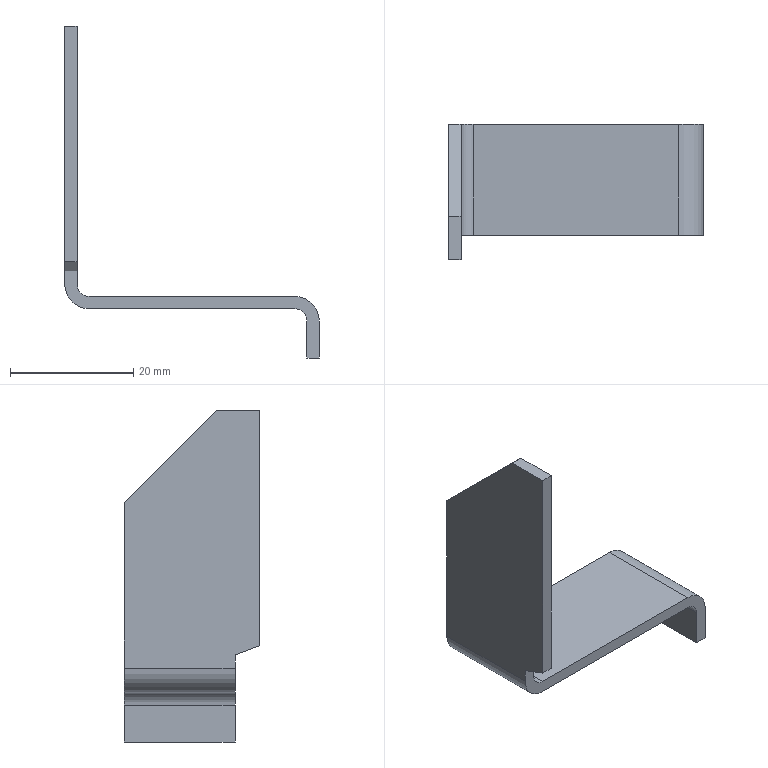Part | NX | features solid 2 | 1 solid | 17 faces | box 41.351 x 22 x 53.937 mm | volume 3353 mm3 | plane 13 | cylinder 4 | commonest cylinder face diameters 4 x2 8 x2
STEP:
#1=CARTESIAN_POINT('',(1112.,-1287.,212.));
#2=VERTEX_POINT('',#1);
#3=CARTESIAN_POINT('',(1112.,-1302.,227.));
#4=VERTEX_POINT('',#3);
#5=CARTESIAN_POINT('',(1112.,-1283.97,208.97));
#6=DIRECTION('',(0.,-0.7071,0.7071));
#7=VECTOR('',#6,1000.);
#8=LINE('',#5,#7);
#9=EDGE_CURVE('',#2,#4,#8,.T.);
#10=ORIENTED_EDGE('',*,*,#9,.F.);
#11=CARTESIAN_POINT('',(1110.,-1287.,212.));
#12=VERTEX_POINT('',#11);
#13=CARTESIAN_POINT('',(1112.,-1287.,212.));
#14=DIRECTION('',(1.,0.,0.));
#15=VECTOR('',#14,1000.);
#16=LINE('',#13,#15);
#17=EDGE_CURVE('',#12,#2,#16,.T.);
#18=ORIENTED_EDGE('',*,*,#17,.F.);
#19=CARTESIAN_POINT('',(1110.,-1302.,227.));
#20=VERTEX_POINT('',#19);
#21=CARTESIAN_POINT('',(1110.,-1302.,227.));
#22=DIRECTION('',(0.,0.7071,-0.7071));
#23=VECTOR('',#22,1000.);
#24=LINE('',#21,#23);
#25=EDGE_CURVE('',#20,#12,#24,.T.);
#26=ORIENTED_EDGE('',*,*,#25,.F.);
#27=CARTESIAN_POINT('',(1112.,-1302.,227.));
#28=DIRECTION('',(-1.,0.,0.));
#29=VECTOR('',#28,1000.);
#30=LINE('',#27,#29);
#31=EDGE_CURVE('',#4,#20,#30,.T.);
#32=ORIENTED_EDGE('',*,*,#31,.F.);
#33=EDGE_LOOP('',(#10,#18,#26,#32));
#34=FACE_BOUND('',#33,.T.);
#35=CARTESIAN_POINT('',(1112.,-1302.,227.));
#36=DIRECTION('',(0.,-0.7071,-0.7071));
#37=DIRECTION('',(0.,0.7071,-0.7071));
#38=AXIS2_PLACEMENT_3D('',#35,#36,#37);
#39=PLANE('',#38);
#40=ADVANCED_FACE('',(#34),#39,.F.);
#41=CARTESIAN_POINT('',(1147.351,-1287.,181.063));
#42=VERTEX_POINT('',#41);
#43=CARTESIAN_POINT('',(1149.351,-1287.,179.063));
#44=VERTEX_POINT('',#43);
#45=CARTESIAN_POINT('',(1147.351,-1287.,179.063));
#46=DIRECTION('',(0.,1.,0.));
#47=DIRECTION('',(0.,0.,1.));
#48=AXIS2_PLACEMENT_3D('',#45,#46,#47);
#49=CIRCLE('',#48,2.);
#50=EDGE_CURVE('',#42,#44,#49,.T.);
#51=ORIENTED_EDGE('',*,*,#50,.T.);
#52=CARTESIAN_POINT('',(1149.351,-1305.,179.063));
#53=VERTEX_POINT('',#52);
#54=CARTESIAN_POINT('',(1149.351,-1267.,179.063));
#55=DIRECTION('',(0.,-1.,0.));
#56=VECTOR('',#55,1000.);
#57=LINE('',#54,#56);
#58=EDGE_CURVE('',#44,#53,#57,.T.);
#59=ORIENTED_EDGE('',*,*,#58,.T.);
#60=CARTESIAN_POINT('',(1147.351,-1305.,181.063));
#61=VERTEX_POINT('',#60);
#62=CARTESIAN_POINT('',(1147.351,-1305.,179.063));
#63=DIRECTION('',(0.,-1.,0.));
#64=DIRECTION('',(0.,0.,1.));
#65=AXIS2_PLACEMENT_3D('',#62,#63,#64);
#66=CIRCLE('',#65,2.);
#67=EDGE_CURVE('',#53,#61,#66,.T.);
#68=ORIENTED_EDGE('',*,*,#67,.T.);
#69=CARTESIAN_POINT('',(1147.351,-1305.,181.063));
#70=DIRECTION('',(0.,1.,0.));
#71=VECTOR('',#70,1000.);
#72=LINE('',#69,#71);
#73=EDGE_CURVE('',#61,#42,#72,.T.);
#74=ORIENTED_EDGE('',*,*,#73,.T.);
#75=EDGE_LOOP('',(#51,#59,#68,#74));
#76=FACE_BOUND('',#75,.T.);
#77=CARTESIAN_POINT('',(1147.351,-1305.,179.063));
#78=DIRECTION('',(0.,1.,0.));
#79=DIRECTION('',(0.,0.,-1.));
#80=AXIS2_PLACEMENT_3D('',#77,#78,#79);
#81=CYLINDRICAL_SURFACE('',#80,2.);
#82=ADVANCED_FACE('',(#76),#81,.F.);
#83=CARTESIAN_POINT('',(1147.351,-1287.,183.063));
#84=VERTEX_POINT('',#83);
#85=CARTESIAN_POINT('',(1151.351,-1287.,179.063));
#86=VERTEX_POINT('',#85);
#87=CARTESIAN_POINT('',(1147.351,-1287.,179.063));
#88=DIRECTION('',(0.,1.,0.));
#89=DIRECTION('',(0.,0.,-1.));
#90=AXIS2_PLACEMENT_3D('',#87,#88,#89);
#91=CIRCLE('',#90,4.);
#92=EDGE_CURVE('',#84,#86,#91,.T.);
#93=ORIENTED_EDGE('',*,*,#92,.F.);
#94=CARTESIAN_POINT('',(1147.351,-1305.,183.063));
#95=VERTEX_POINT('',#94);
#96=CARTESIAN_POINT('',(1147.351,-1305.,183.063));
#97=DIRECTION('',(0.,1.,0.));
#98=VECTOR('',#97,1000.);
#99=LINE('',#96,#98);
#100=EDGE_CURVE('',#95,#84,#99,.T.);
#101=ORIENTED_EDGE('',*,*,#100,.F.);
#102=CARTESIAN_POINT('',(1151.351,-1305.,179.063));
#103=VERTEX_POINT('',#102);
#104=CARTESIAN_POINT('',(1147.351,-1305.,179.063));
#105=DIRECTION('',(0.,-1.,0.));
#106=DIRECTION('',(0.,0.,-1.));
#107=AXIS2_PLACEMENT_3D('',#104,#105,#106);
#108=CIRCLE('',#107,4.);
#109=EDGE_CURVE('',#103,#95,#108,.T.);
#110=ORIENTED_EDGE('',*,*,#109,.F.);
#111=CARTESIAN_POINT('',(1151.351,-1267.,179.063));
#112=DIRECTION('',(0.,-1.,0.));
#113=VECTOR('',#112,1000.);
#114=LINE('',#111,#113);
#115=EDGE_CURVE('',#86,#103,#114,.T.);
#116=ORIENTED_EDGE('',*,*,#115,.F.);
#117=EDGE_LOOP('',(#93,#101,#110,#116));
#118=FACE_BOUND('',#117,.T.);
#119=CARTESIAN_POINT('',(1147.351,-1305.,179.063));
#120=DIRECTION('',(0.,1.,0.));
#121=DIRECTION('',(0.,0.,-1.));
#122=AXIS2_PLACEMENT_3D('',#119,#120,#121);
#123=CYLINDRICAL_SURFACE('',#122,4.);
#124=ADVANCED_FACE('',(#118),#123,.T.);
#125=CARTESIAN_POINT('',(1149.351,-1305.,173.063));
#126=VERTEX_POINT('',#125);
#127=CARTESIAN_POINT('',(1149.351,-1287.,173.063));
#128=VERTEX_POINT('',#127);
#129=CARTESIAN_POINT('',(1149.351,-1305.,173.063));
#130=DIRECTION('',(0.,1.,0.));
#131=VECTOR('',#130,1000.);
#132=LINE('',#129,#131);
#133=EDGE_CURVE('',#126,#128,#132,.T.);
#134=ORIENTED_EDGE('',*,*,#133,.T.);
#135=CARTESIAN_POINT('',(1151.351,-1287.,173.063));
#136=VERTEX_POINT('',#135);
#137=CARTESIAN_POINT('',(1151.351,-1287.,173.063));
#138=DIRECTION('',(-1.,0.,0.));
#139=VECTOR('',#138,1000.);
#140=LINE('',#137,#139);
#141=EDGE_CURVE('',#136,#128,#140,.T.);
#142=ORIENTED_EDGE('',*,*,#141,.F.);
#143=CARTESIAN_POINT('',(1151.351,-1305.,173.063));
#144=VERTEX_POINT('',#143);
#145=CARTESIAN_POINT('',(1151.351,-1305.,173.063));
#146=DIRECTION('',(0.,1.,0.));
#147=VECTOR('',#146,1000.);
#148=LINE('',#145,#147);
#149=EDGE_CURVE('',#144,#136,#148,.T.);
#150=ORIENTED_EDGE('',*,*,#149,.F.);
#151=CARTESIAN_POINT('',(1151.351,-1305.,173.063));
#152=DIRECTION('',(-1.,0.,0.));
#153=VECTOR('',#152,1000.);
#154=LINE('',#151,#153);
#155=EDGE_CURVE('',#144,#126,#154,.T.);
#156=ORIENTED_EDGE('',*,*,#155,.T.);
#157=EDGE_LOOP('',(#134,#142,#150,#156));
#158=FACE_BOUND('',#157,.T.);
#159=CARTESIAN_POINT('',(1151.351,-1305.,173.063));
#160=DIRECTION('',(0.,0.,1.));
#161=DIRECTION('',(1.,0.,0.));
#162=AXIS2_PLACEMENT_3D('',#159,#160,#161);
#163=PLANE('',#162);
#164=ADVANCED_FACE('',(#158),#163,.F.);
#165=ORIENTED_EDGE('',*,*,#58,.F.);
#166=CARTESIAN_POINT('',(1149.351,-1287.,181.341));
#167=DIRECTION('',(0.,0.,1.));
#168=VECTOR('',#167,1000.);
#169=LINE('',#166,#168);
#170=EDGE_CURVE('',#128,#44,#169,.T.);
#171=ORIENTED_EDGE('',*,*,#170,.F.);
#172=ORIENTED_EDGE('',*,*,#133,.F.);
#173=CARTESIAN_POINT('',(1149.351,-1305.,181.341));
#174=DIRECTION('',(0.,0.,-1.));
#175=VECTOR('',#174,1000.);
#176=LINE('',#173,#175);
#177=EDGE_CURVE('',#53,#126,#176,.T.);
#178=ORIENTED_EDGE('',*,*,#177,.F.);
#179=EDGE_LOOP('',(#165,#171,#172,#178));
#180=FACE_BOUND('',#179,.T.);
#181=CARTESIAN_POINT('',(1149.351,-1555.,-62.061));
#182=DIRECTION('',(1.,0.,0.));
#183=DIRECTION('',(0.,0.,1.));
#184=AXIS2_PLACEMENT_3D('',#181,#182,#183);
#185=PLANE('',#184);
#186=ADVANCED_FACE('',(#180),#185,.F.);
#187=CARTESIAN_POINT('',(1151.351,-1287.,181.341));
#188=DIRECTION('',(0.,0.,1.));
#189=VECTOR('',#188,1000.);
#190=LINE('',#187,#189);
#191=EDGE_CURVE('',#136,#86,#190,.T.);
#192=ORIENTED_EDGE('',*,*,#191,.T.);
#193=ORIENTED_EDGE('',*,*,#115,.T.);
#194=CARTESIAN_POINT('',(1151.351,-1305.,181.341));
#195=DIRECTION('',(0.,0.,-1.));
#196=VECTOR('',#195,1000.);
#197=LINE('',#194,#196);
#198=EDGE_CURVE('',#103,#144,#197,.T.);
#199=ORIENTED_EDGE('',*,*,#198,.T.);
#200=ORIENTED_EDGE('',*,*,#149,.T.);
#201=EDGE_LOOP('',(#192,#193,#199,#200));
#202=FACE_BOUND('',#201,.T.);
#203=CARTESIAN_POINT('',(1151.351,-1555.,-62.061));
#204=DIRECTION('',(1.,0.,0.));
#205=DIRECTION('',(0.,0.,1.));
#206=AXIS2_PLACEMENT_3D('',#203,#204,#205);
#207=PLANE('',#206);
#208=ADVANCED_FACE('',(#202),#207,.T.);
#209=CARTESIAN_POINT('',(1112.,-1287.,185.063));
#210=VERTEX_POINT('',#209);
#211=CARTESIAN_POINT('',(1112.,-1305.,185.063));
#212=VERTEX_POINT('',#211);
#213=CARTESIAN_POINT('',(1112.,-1267.,185.063));
#214=DIRECTION('',(0.,-1.,0.));
#215=VECTOR('',#214,1000.);
#216=LINE('',#213,#215);
#217=EDGE_CURVE('',#210,#212,#216,.T.);
#218=ORIENTED_EDGE('',*,*,#217,.T.);
#219=CARTESIAN_POINT('',(1114.,-1305.,183.063));
#220=VERTEX_POINT('',#219);
#221=CARTESIAN_POINT('',(1114.,-1305.,185.063));
#222=DIRECTION('',(0.,-1.,0.));
#223=DIRECTION('',(0.,0.,-1.));
#224=AXIS2_PLACEMENT_3D('',#221,#222,#223);
#225=CIRCLE('',#224,2.);
#226=EDGE_CURVE('',#212,#220,#225,.T.);
#227=ORIENTED_EDGE('',*,*,#226,.T.);
#228=CARTESIAN_POINT('',(1114.,-1287.,183.063));
#229=VERTEX_POINT('',#228);
#230=CARTESIAN_POINT('',(1114.,-1305.,183.063));
#231=DIRECTION('',(0.,1.,0.));
#232=VECTOR('',#231,1000.);
#233=LINE('',#230,#232);
#234=EDGE_CURVE('',#220,#229,#233,.T.);
#235=ORIENTED_EDGE('',*,*,#234,.T.);
#236=CARTESIAN_POINT('',(1114.,-1287.,185.063));
#237=DIRECTION('',(0.,1.,0.));
#238=DIRECTION('',(0.,0.,-1.));
#239=AXIS2_PLACEMENT_3D('',#236,#237,#238);
#240=CIRCLE('',#239,2.);
#241=EDGE_CURVE('',#229,#210,#240,.T.);
#242=ORIENTED_EDGE('',*,*,#241,.T.);
#243=EDGE_LOOP('',(#218,#227,#235,#242));
#244=FACE_BOUND('',#243,.T.);
#245=CARTESIAN_POINT('',(1114.,-1267.,185.063));
#246=DIRECTION('',(0.,-1.,0.));
#247=DIRECTION('',(1.,0.,0.));
#248=AXIS2_PLACEMENT_3D('',#245,#246,#247);
#249=CYLINDRICAL_SURFACE('',#248,2.);
#250=ADVANCED_FACE('',(#244),#249,.F.);
#251=CARTESIAN_POINT('',(1110.,-1287.,185.063));
#252=VERTEX_POINT('',#251);
#253=CARTESIAN_POINT('',(1110.,-1305.,185.063));
#254=VERTEX_POINT('',#253);
#255=CARTESIAN_POINT('',(1110.,-1267.,185.063));
#256=DIRECTION('',(0.,-1.,0.));
#257=VECTOR('',#256,1000.);
#258=LINE('',#255,#257);
#259=EDGE_CURVE('',#252,#254,#258,.T.);
#260=ORIENTED_EDGE('',*,*,#259,.F.);
#261=CARTESIAN_POINT('',(1114.,-1287.,181.063));
#262=VERTEX_POINT('',#261);
#263=CARTESIAN_POINT('',(1114.,-1287.,185.063));
#264=DIRECTION('',(0.,1.,0.));
#265=DIRECTION('',(1.,0.,0.));
#266=AXIS2_PLACEMENT_3D('',#263,#264,#265);
#267=CIRCLE('',#266,4.);
#268=EDGE_CURVE('',#262,#252,#267,.T.);
#269=ORIENTED_EDGE('',*,*,#268,.F.);
#270=CARTESIAN_POINT('',(1114.,-1305.,181.063));
#271=VERTEX_POINT('',#270);
#272=CARTESIAN_POINT('',(1114.,-1305.,181.063));
#273=DIRECTION('',(0.,1.,0.));
#274=VECTOR('',#273,1000.);
#275=LINE('',#272,#274);
#276=EDGE_CURVE('',#271,#262,#275,.T.);
#277=ORIENTED_EDGE('',*,*,#276,.F.);
#278=CARTESIAN_POINT('',(1114.,-1305.,185.063));
#279=DIRECTION('',(0.,-1.,0.));
#280=DIRECTION('',(1.,0.,0.));
#281=AXIS2_PLACEMENT_3D('',#278,#279,#280);
#282=CIRCLE('',#281,4.);
#283=EDGE_CURVE('',#254,#271,#282,.T.);
#284=ORIENTED_EDGE('',*,*,#283,.F.);
#285=EDGE_LOOP('',(#260,#269,#277,#284));
#286=FACE_BOUND('',#285,.T.);
#287=CARTESIAN_POINT('',(1114.,-1267.,185.063));
#288=DIRECTION('',(0.,-1.,0.));
#289=DIRECTION('',(1.,0.,0.));
#290=AXIS2_PLACEMENT_3D('',#287,#288,#289);
#291=CYLINDRICAL_SURFACE('',#290,4.);
#292=ADVANCED_FACE('',(#286),#291,.T.);
#293=ORIENTED_EDGE('',*,*,#73,.F.);
#294=CARTESIAN_POINT('',(1111.722,-1305.,181.063));
#295=DIRECTION('',(-1.,0.,0.));
#296=VECTOR('',#295,1000.);
#297=LINE('',#294,#296);
#298=EDGE_CURVE('',#61,#271,#297,.T.);
#299=ORIENTED_EDGE('',*,*,#298,.T.);
#300=ORIENTED_EDGE('',*,*,#276,.T.);
#301=CARTESIAN_POINT('',(1111.722,-1287.,181.063));
#302=DIRECTION('',(1.,0.,0.));
#303=VECTOR('',#302,1000.);
#304=LINE('',#301,#303);
#305=EDGE_CURVE('',#262,#42,#304,.T.);
#306=ORIENTED_EDGE('',*,*,#305,.T.);
#307=EDGE_LOOP('',(#293,#299,#300,#306));
#308=FACE_BOUND('',#307,.T.);
#309=CARTESIAN_POINT('',(1110.,-1555.,181.063));
#310=DIRECTION('',(0.,0.,-1.));
#311=DIRECTION('',(0.,-1.,0.));
#312=AXIS2_PLACEMENT_3D('',#309,#310,#311);
#313=PLANE('',#312);
#314=ADVANCED_FACE('',(#308),#313,.T.);
#315=CARTESIAN_POINT('',(1112.,-1287.,227.));
#316=DIRECTION('',(0.,0.,1.));
#317=VECTOR('',#316,1000.);
#318=LINE('',#315,#317);
#319=EDGE_CURVE('',#210,#2,#318,.T.);
#320=ORIENTED_EDGE('',*,*,#319,.T.);
#321=ORIENTED_EDGE('',*,*,#9,.T.);
#322=CARTESIAN_POINT('',(1112.,-1309.,227.));
#323=VERTEX_POINT('',#322);
#324=CARTESIAN_POINT('',(1112.,-1309.,227.));
#325=DIRECTION('',(0.,-1.,0.));
#326=VECTOR('',#325,1000.);
#327=LINE('',#324,#326);
#328=EDGE_CURVE('',#4,#323,#327,.T.);
#329=ORIENTED_EDGE('',*,*,#328,.T.);
#330=CARTESIAN_POINT('',(1112.,-1309.,188.716));
#331=VERTEX_POINT('',#330);
#332=CARTESIAN_POINT('',(1112.,-1309.,188.716));
#333=DIRECTION('',(0.,0.,-1.));
#334=VECTOR('',#333,1000.);
#335=LINE('',#332,#334);
#336=EDGE_CURVE('',#323,#331,#335,.T.);
#337=ORIENTED_EDGE('',*,*,#336,.T.);
#338=CARTESIAN_POINT('',(1112.,-1305.,187.22));
#339=VERTEX_POINT('',#338);
#340=CARTESIAN_POINT('',(1112.,-1309.,188.716));
#341=DIRECTION('',(0.,0.9366,-0.3504));
#342=VECTOR('',#341,1000.);
#343=LINE('',#340,#342);
#344=EDGE_CURVE('',#331,#339,#343,.T.);
#345=ORIENTED_EDGE('',*,*,#344,.T.);
#346=CARTESIAN_POINT('',(1112.,-1305.,187.22));
#347=DIRECTION('',(0.,0.,-1.));
#348=VECTOR('',#347,1000.);
#349=LINE('',#346,#348);
#350=EDGE_CURVE('',#339,#212,#349,.T.);
#351=ORIENTED_EDGE('',*,*,#350,.T.);
#352=ORIENTED_EDGE('',*,*,#217,.F.);
#353=EDGE_LOOP('',(#320,#321,#329,#337,#345,#351,#352));
#354=FACE_BOUND('',#353,.T.);
#355=CARTESIAN_POINT('',(1112.,-1555.,-62.061));
#356=DIRECTION('',(1.,0.,0.));
#357=DIRECTION('',(0.,0.,1.));
#358=AXIS2_PLACEMENT_3D('',#355,#356,#357);
#359=PLANE('',#358);
#360=ADVANCED_FACE('',(#354),#359,.T.);
#361=CARTESIAN_POINT('',(1110.,-1309.,188.716));
#362=VERTEX_POINT('',#361);
#363=CARTESIAN_POINT('',(1110.,-1305.,187.22));
#364=VERTEX_POINT('',#363);
#365=CARTESIAN_POINT('',(1110.,-1309.,188.716));
#366=DIRECTION('',(0.,0.9366,-0.3504));
#367=VECTOR('',#366,1000.);
#368=LINE('',#365,#367);
#369=EDGE_CURVE('',#362,#364,#368,.T.);
#370=ORIENTED_EDGE('',*,*,#369,.T.);
#371=CARTESIAN_POINT('',(1112.,-1305.,187.22));
#372=DIRECTION('',(-1.,0.,0.));
#373=VECTOR('',#372,1000.);
#374=LINE('',#371,#373);
#375=EDGE_CURVE('',#339,#364,#374,.T.);
#376=ORIENTED_EDGE('',*,*,#375,.F.);
#377=ORIENTED_EDGE('',*,*,#344,.F.);
#378=CARTESIAN_POINT('',(1112.,-1309.,188.716));
#379=DIRECTION('',(-1.,0.,0.));
#380=VECTOR('',#379,1000.);
#381=LINE('',#378,#380);
#382=EDGE_CURVE('',#331,#362,#381,.T.);
#383=ORIENTED_EDGE('',*,*,#382,.T.);
#384=EDGE_LOOP('',(#370,#376,#377,#383));
#385=FACE_BOUND('',#384,.T.);
#386=CARTESIAN_POINT('',(1112.,-1309.,188.716));
#387=DIRECTION('',(0.,0.3504,0.9366));
#388=DIRECTION('',(1.,0.,0.));
#389=AXIS2_PLACEMENT_3D('',#386,#387,#388);
#390=PLANE('',#389);
#391=ADVANCED_FACE('',(#385),#390,.F.);
#392=CARTESIAN_POINT('',(1110.,-1309.,227.));
#393=VERTEX_POINT('',#392);
#394=CARTESIAN_POINT('',(1110.,-1309.,188.716));
#395=DIRECTION('',(0.,0.,-1.));
#396=VECTOR('',#395,1000.);
#397=LINE('',#394,#396);
#398=EDGE_CURVE('',#393,#362,#397,.T.);
#399=ORIENTED_EDGE('',*,*,#398,.T.);
#400=ORIENTED_EDGE('',*,*,#382,.F.);
#401=ORIENTED_EDGE('',*,*,#336,.F.);
#402=CARTESIAN_POINT('',(1112.,-1309.,227.));
#403=DIRECTION('',(-1.,0.,0.));
#404=VECTOR('',#403,1000.);
#405=LINE('',#402,#404);
#406=EDGE_CURVE('',#323,#393,#405,.T.);
#407=ORIENTED_EDGE('',*,*,#406,.T.);
#408=EDGE_LOOP('',(#399,#400,#401,#407));
#409=FACE_BOUND('',#408,.T.);
#410=CARTESIAN_POINT('',(1112.,-1309.,188.716));
#411=DIRECTION('',(0.,1.,0.));
#412=DIRECTION('',(0.,0.,-1.));
#413=AXIS2_PLACEMENT_3D('',#410,#411,#412);
#414=PLANE('',#413);
#415=ADVANCED_FACE('',(#409),#414,.F.);
#416=ORIENTED_EDGE('',*,*,#328,.F.);
#417=ORIENTED_EDGE('',*,*,#31,.T.);
#418=CARTESIAN_POINT('',(1110.,-1309.,227.));
#419=DIRECTION('',(0.,-1.,0.));
#420=VECTOR('',#419,1000.);
#421=LINE('',#418,#420);
#422=EDGE_CURVE('',#20,#393,#421,.T.);
#423=ORIENTED_EDGE('',*,*,#422,.T.);
#424=ORIENTED_EDGE('',*,*,#406,.F.);
#425=EDGE_LOOP('',(#416,#417,#423,#424));
#426=FACE_BOUND('',#425,.T.);
#427=CARTESIAN_POINT('',(1112.,-1309.,227.));
#428=DIRECTION('',(0.,0.,-1.));
#429=DIRECTION('',(0.,-1.,0.));
#430=AXIS2_PLACEMENT_3D('',#427,#428,#429);
#431=PLANE('',#430);
#432=ADVANCED_FACE('',(#426),#431,.F.);
#433=ORIENTED_EDGE('',*,*,#422,.F.);
#434=ORIENTED_EDGE('',*,*,#25,.T.);
#435=CARTESIAN_POINT('',(1110.,-1287.,227.));
#436=DIRECTION('',(0.,0.,1.));
#437=VECTOR('',#436,1000.);
#438=LINE('',#435,#437);
#439=EDGE_CURVE('',#252,#12,#438,.T.);
#440=ORIENTED_EDGE('',*,*,#439,.F.);
#441=ORIENTED_EDGE('',*,*,#259,.T.);
#442=CARTESIAN_POINT('',(1110.,-1305.,187.22));
#443=DIRECTION('',(0.,0.,-1.));
#444=VECTOR('',#443,1000.);
#445=LINE('',#442,#444);
#446=EDGE_CURVE('',#364,#254,#445,.T.);
#447=ORIENTED_EDGE('',*,*,#446,.F.);
#448=ORIENTED_EDGE('',*,*,#369,.F.);
#449=ORIENTED_EDGE('',*,*,#398,.F.);
#450=EDGE_LOOP('',(#433,#434,#440,#441,#447,#448,#449));
#451=FACE_BOUND('',#450,.T.);
#452=CARTESIAN_POINT('',(1110.,-1555.,-62.061));
#453=DIRECTION('',(1.,0.,0.));
#454=DIRECTION('',(0.,0.,1.));
#455=AXIS2_PLACEMENT_3D('',#452,#453,#454);
#456=PLANE('',#455);
#457=ADVANCED_FACE('',(#451),#456,.F.);
#458=CARTESIAN_POINT('',(1111.722,-1305.,183.063));
#459=DIRECTION('',(-1.,0.,0.));
#460=VECTOR('',#459,1000.);
#461=LINE('',#458,#460);
#462=EDGE_CURVE('',#95,#220,#461,.T.);
#463=ORIENTED_EDGE('',*,*,#462,.F.);
#464=ORIENTED_EDGE('',*,*,#100,.T.);
#465=CARTESIAN_POINT('',(1111.722,-1287.,183.063));
#466=DIRECTION('',(1.,0.,0.));
#467=VECTOR('',#466,1000.);
#468=LINE('',#465,#467);
#469=EDGE_CURVE('',#229,#84,#468,.T.);
#470=ORIENTED_EDGE('',*,*,#469,.F.);
#471=ORIENTED_EDGE('',*,*,#234,.F.);
#472=EDGE_LOOP('',(#463,#464,#470,#471));
#473=FACE_BOUND('',#472,.T.);
#474=CARTESIAN_POINT('',(1110.,-1555.,183.063));
#475=DIRECTION('',(0.,0.,-1.));
#476=DIRECTION('',(0.,-1.,0.));
#477=AXIS2_PLACEMENT_3D('',#474,#475,#476);
#478=PLANE('',#477);
#479=ADVANCED_FACE('',(#473),#478,.F.);
#480=ORIENTED_EDGE('',*,*,#298,.F.);
#481=ORIENTED_EDGE('',*,*,#67,.F.);
#482=ORIENTED_EDGE('',*,*,#177,.T.);
#483=ORIENTED_EDGE('',*,*,#155,.F.);
#484=ORIENTED_EDGE('',*,*,#198,.F.);
#485=ORIENTED_EDGE('',*,*,#109,.T.);
#486=ORIENTED_EDGE('',*,*,#462,.T.);
#487=ORIENTED_EDGE('',*,*,#226,.F.);
#488=ORIENTED_EDGE('',*,*,#350,.F.);
#489=ORIENTED_EDGE('',*,*,#375,.T.);
#490=ORIENTED_EDGE('',*,*,#446,.T.);
#491=ORIENTED_EDGE('',*,*,#283,.T.);
#492=EDGE_LOOP('',(#480,#481,#482,#483,#484,#485,#486,#487,#488,#489,#490,#491));
#493=FACE_BOUND('',#492,.T.);
#494=CARTESIAN_POINT('',(1112.,-1305.,187.22));
#495=DIRECTION('',(0.,1.,0.));
#496=DIRECTION('',(0.,0.,-1.));
#497=AXIS2_PLACEMENT_3D('',#494,#495,#496);
#498=PLANE('',#497);
#499=ADVANCED_FACE('',(#493),#498,.F.);
#500=ORIENTED_EDGE('',*,*,#439,.T.);
#501=ORIENTED_EDGE('',*,*,#17,.T.);
#502=ORIENTED_EDGE('',*,*,#319,.F.);
#503=ORIENTED_EDGE('',*,*,#241,.F.);
#504=ORIENTED_EDGE('',*,*,#469,.T.);
#505=ORIENTED_EDGE('',*,*,#92,.T.);
#506=ORIENTED_EDGE('',*,*,#191,.F.);
#507=ORIENTED_EDGE('',*,*,#141,.T.);
#508=ORIENTED_EDGE('',*,*,#170,.T.);
#509=ORIENTED_EDGE('',*,*,#50,.F.);
#510=ORIENTED_EDGE('',*,*,#305,.F.);
#511=ORIENTED_EDGE('',*,*,#268,.T.);
#512=EDGE_LOOP('',(#500,#501,#502,#503,#504,#505,#506,#507,#508,#509,#510,#511));
#513=FACE_BOUND('',#512,.T.);
#514=CARTESIAN_POINT('',(1112.,-1287.,227.));
#515=DIRECTION('',(0.,-1.,0.));
#516=DIRECTION('',(0.,0.,-1.));
#517=AXIS2_PLACEMENT_3D('',#514,#515,#516);
#518=PLANE('',#517);
#519=ADVANCED_FACE('',(#513),#518,.F.);
#520=CLOSED_SHELL('',(#40,#82,#124,#164,#186,#208,#250,#292,#314,#360,#391,#415,#432,#457,#479,#499,#519));
#521=MANIFOLD_SOLID_BREP('',#520);
#522=(LENGTH_UNIT()NAMED_UNIT(*)SI_UNIT(.MILLI.,.METRE.));
#523=UNCERTAINTY_MEASURE_WITH_UNIT(LENGTH_MEASURE(0.00001),#522,'','');
#524=(NAMED_UNIT(*)PLANE_ANGLE_UNIT()SI_UNIT($,.RADIAN.));
#525=(NAMED_UNIT(*)SI_UNIT($,.STERADIAN.)SOLID_ANGLE_UNIT());
#526=(GEOMETRIC_REPRESENTATION_CONTEXT(3)GLOBAL_UNCERTAINTY_ASSIGNED_CONTEXT((#523))GLOBAL_UNIT_ASSIGNED_CONTEXT((#522,#524,#525))REPRESENTATION_CONTEXT('',''));
#527=ADVANCED_BREP_SHAPE_REPRESENTATION('',(#521),#526);